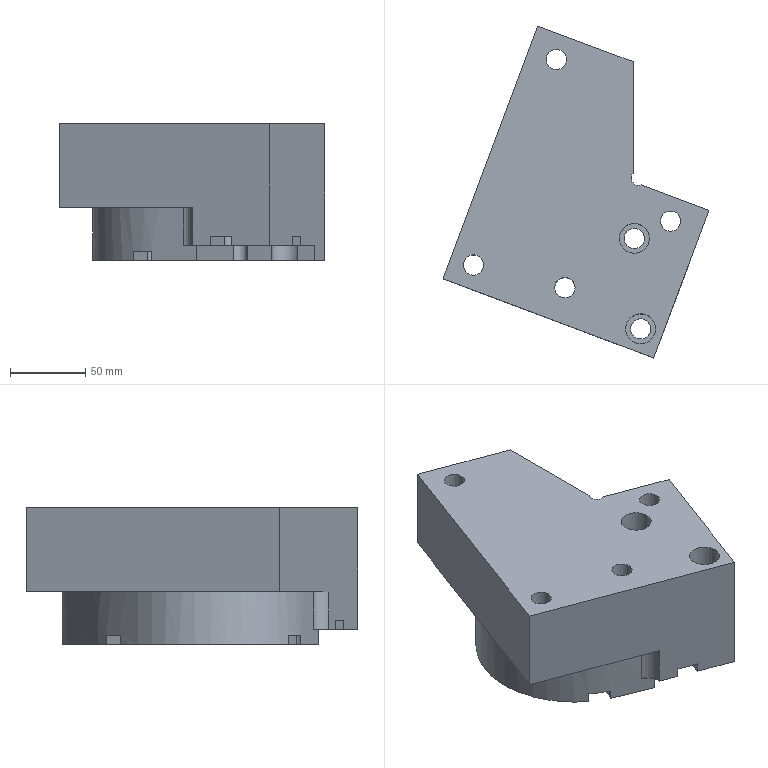Part | NX | features 8 2 | 1 solid | 68 faces | box 177.272 x 221.132 x 91 mm | volume 1669276 mm3 | plane 31 | cylinder 29 | cone 7 | spline 1 | commonest cylinder face diameters 15 x7 20 x7 13.5 x6 8.5 x3 5.199 x2 5.2 x2